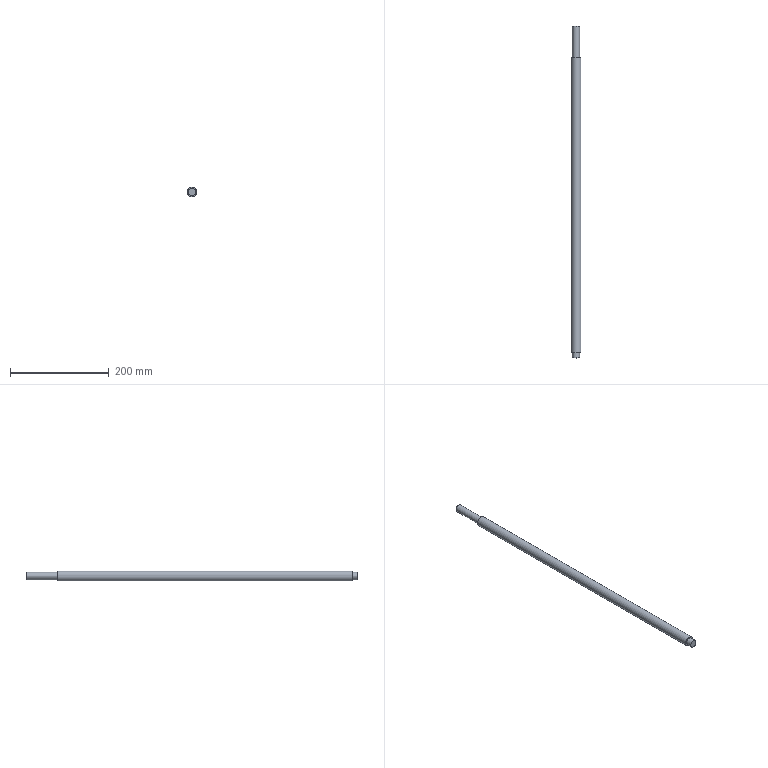Part | STEP file | tulunzhou | 1 solid | 7 faces | box 20 x 672 x 20 mm | volume 200669 mm3 | plane 4 | cylinder 3 | commonest cylinder face diameters 15 x2 20 x1
STEP:
#1=CARTESIAN_POINT('',(0.,0.,0.));
#2=DIRECTION('',(0.,0.,1.));
#3=DIRECTION('',(1.,0.,0.));
#4=AXIS2_PLACEMENT_3D('',#1,#2,#3);
#5=CARTESIAN_POINT('',(0.,12.,7.5));
#6=VERTEX_POINT('',#5);
#7=CARTESIAN_POINT('',(0.,12.,0.));
#8=DIRECTION('',(0.,1.,0.));
#9=DIRECTION('',(0.,0.,1.));
#10=AXIS2_PLACEMENT_3D('',#7,#8,#9);
#11=CIRCLE('',#10,7.5);
#12=CARTESIAN_POINT('',(0.,12.,0.));
#13=DIRECTION('',(0.,-1.,0.));
#14=DIRECTION('',(0.,0.,-1.));
#15=AXIS2_PLACEMENT_3D('',#12,#13,#14);
#16=CYLINDRICAL_SURFACE('',#15,7.5);
#17=CARTESIAN_POINT('',(9.425,0.));
#18=DIRECTION('',(-1.,0.));
#19=VECTOR('',#18,1.);
#20=LINE('',#17,#19);
#21=(GEOMETRIC_REPRESENTATION_CONTEXT(2)PARAMETRIC_REPRESENTATION_CONTEXT()REPRESENTATION_CONTEXT('',''));
#22=DEFINITIONAL_REPRESENTATION('',(#20),#21);
#23=PCURVE('',#16,#22);
#24=CARTESIAN_POINT('',(0.,12.,0.));
#25=DIRECTION('',(0.,1.,0.));
#26=DIRECTION('',(0.,0.,1.));
#27=AXIS2_PLACEMENT_3D('',#24,#25,#26);
#28=PLANE('',#27);
#29=CARTESIAN_POINT('',(0.,0.));
#30=DIRECTION('',(1.,0.));
#31=AXIS2_PLACEMENT_2D('',#29,#30);
#32=CIRCLE('',#31,7.5);
#33=(GEOMETRIC_REPRESENTATION_CONTEXT(2)PARAMETRIC_REPRESENTATION_CONTEXT()REPRESENTATION_CONTEXT('',''));
#34=DEFINITIONAL_REPRESENTATION('',(#32),#33);
#35=PCURVE('',#28,#34);
#36=SURFACE_CURVE('',#11,(#23,#35),.PCURVE_S1.);
#37=EDGE_CURVE('',#6,#6,#36,.T.);
#38=ORIENTED_EDGE('',*,*,#37,.F.);
#39=CARTESIAN_POINT('',(0.,0.,7.5));
#40=VERTEX_POINT('',#39);
#41=CARTESIAN_POINT('',(0.,12.,7.5));
#42=CARTESIAN_POINT('',(0.,0.,7.5));
#43=B_SPLINE_CURVE_WITH_KNOTS('',1,(#41,#42),.UNSPECIFIED.,.F.,.F.,(2,2),(0.,12.),.PIECEWISE_BEZIER_KNOTS.);
#44=CARTESIAN_POINT('',(9.425,0.));
#45=DIRECTION('',(0.,1.));
#46=VECTOR('',#45,1.);
#47=LINE('',#44,#46);
#48=(GEOMETRIC_REPRESENTATION_CONTEXT(2)PARAMETRIC_REPRESENTATION_CONTEXT()REPRESENTATION_CONTEXT('',''));
#49=DEFINITIONAL_REPRESENTATION('',(#47),#48);
#50=PCURVE('',#16,#49);
#51=CARTESIAN_POINT('',(3.142,0.));
#52=DIRECTION('',(0.,1.));
#53=VECTOR('',#52,1.);
#54=LINE('',#51,#53);
#55=(GEOMETRIC_REPRESENTATION_CONTEXT(2)PARAMETRIC_REPRESENTATION_CONTEXT()REPRESENTATION_CONTEXT('',''));
#56=DEFINITIONAL_REPRESENTATION('',(#54),#55);
#57=PCURVE('',#16,#56);
#58=SEAM_CURVE('',#43,(#50,#57),.PCURVE_S1.);
#59=EDGE_CURVE('',#6,#40,#58,.T.);
#60=ORIENTED_EDGE('',*,*,#59,.T.);
#61=CARTESIAN_POINT('',(0.,0.,0.));
#62=DIRECTION('',(0.,1.,0.));
#63=DIRECTION('',(0.,0.,1.));
#64=AXIS2_PLACEMENT_3D('',#61,#62,#63);
#65=CIRCLE('',#64,7.5);
#66=CARTESIAN_POINT('',(9.425,12.));
#67=DIRECTION('',(-1.,0.));
#68=VECTOR('',#67,1.);
#69=LINE('',#66,#68);
#70=(GEOMETRIC_REPRESENTATION_CONTEXT(2)PARAMETRIC_REPRESENTATION_CONTEXT()REPRESENTATION_CONTEXT('',''));
#71=DEFINITIONAL_REPRESENTATION('',(#69),#70);
#72=PCURVE('',#16,#71);
#73=CARTESIAN_POINT('',(0.,0.,0.));
#74=DIRECTION('',(0.,1.,0.));
#75=DIRECTION('',(0.,0.,1.));
#76=AXIS2_PLACEMENT_3D('',#73,#74,#75);
#77=PLANE('',#76);
#78=CARTESIAN_POINT('',(0.,0.));
#79=DIRECTION('',(1.,0.));
#80=AXIS2_PLACEMENT_2D('',#78,#79);
#81=CIRCLE('',#80,7.5);
#82=(GEOMETRIC_REPRESENTATION_CONTEXT(2)PARAMETRIC_REPRESENTATION_CONTEXT()REPRESENTATION_CONTEXT('',''));
#83=DEFINITIONAL_REPRESENTATION('',(#81),#82);
#84=PCURVE('',#77,#83);
#85=SURFACE_CURVE('',#65,(#72,#84),.PCURVE_S1.);
#86=EDGE_CURVE('',#40,#40,#85,.T.);
#87=ORIENTED_EDGE('',*,*,#86,.T.);
#88=ORIENTED_EDGE('',*,*,#59,.F.);
#89=EDGE_LOOP('',(#38,#60,#87,#88));
#90=FACE_BOUND('',#89,.T.);
#91=ADVANCED_FACE('',(#90),#16,.T.);
#92=ORIENTED_EDGE('',*,*,#86,.F.);
#93=EDGE_LOOP('',(#92));
#94=FACE_BOUND('',#93,.T.);
#95=ADVANCED_FACE('',(#94),#77,.F.);
#96=CARTESIAN_POINT('',(0.,608.,10.));
#97=VERTEX_POINT('',#96);
#98=CARTESIAN_POINT('',(0.,608.,0.));
#99=DIRECTION('',(0.,1.,0.));
#100=DIRECTION('',(0.,0.,1.));
#101=AXIS2_PLACEMENT_3D('',#98,#99,#100);
#102=CIRCLE('',#101,10.);
#103=CARTESIAN_POINT('',(0.,608.,0.));
#104=DIRECTION('',(0.,-1.,0.));
#105=DIRECTION('',(0.,0.,-1.));
#106=AXIS2_PLACEMENT_3D('',#103,#104,#105);
#107=CYLINDRICAL_SURFACE('',#106,10.);
#108=CARTESIAN_POINT('',(9.425,0.));
#109=DIRECTION('',(-1.,0.));
#110=VECTOR('',#109,1.);
#111=LINE('',#108,#110);
#112=(GEOMETRIC_REPRESENTATION_CONTEXT(2)PARAMETRIC_REPRESENTATION_CONTEXT()REPRESENTATION_CONTEXT('',''));
#113=DEFINITIONAL_REPRESENTATION('',(#111),#112);
#114=PCURVE('',#107,#113);
#115=CARTESIAN_POINT('',(0.,608.,0.));
#116=DIRECTION('',(0.,1.,0.));
#117=DIRECTION('',(0.,0.,1.));
#118=AXIS2_PLACEMENT_3D('',#115,#116,#117);
#119=PLANE('',#118);
#120=CARTESIAN_POINT('',(0.,0.));
#121=DIRECTION('',(1.,0.));
#122=AXIS2_PLACEMENT_2D('',#120,#121);
#123=CIRCLE('',#122,10.);
#124=(GEOMETRIC_REPRESENTATION_CONTEXT(2)PARAMETRIC_REPRESENTATION_CONTEXT()REPRESENTATION_CONTEXT('',''));
#125=DEFINITIONAL_REPRESENTATION('',(#123),#124);
#126=PCURVE('',#119,#125);
#127=SURFACE_CURVE('',#102,(#114,#126),.PCURVE_S1.);
#128=EDGE_CURVE('',#97,#97,#127,.T.);
#129=ORIENTED_EDGE('',*,*,#128,.F.);
#130=CARTESIAN_POINT('',(0.,12.,10.));
#131=VERTEX_POINT('',#130);
#132=CARTESIAN_POINT('',(0.,608.,10.));
#133=CARTESIAN_POINT('',(0.,12.,10.));
#134=B_SPLINE_CURVE_WITH_KNOTS('',1,(#132,#133),.UNSPECIFIED.,.F.,.F.,(2,2),(0.,596.),.PIECEWISE_BEZIER_KNOTS.);
#135=CARTESIAN_POINT('',(9.425,0.));
#136=DIRECTION('',(0.,1.));
#137=VECTOR('',#136,1.);
#138=LINE('',#135,#137);
#139=(GEOMETRIC_REPRESENTATION_CONTEXT(2)PARAMETRIC_REPRESENTATION_CONTEXT()REPRESENTATION_CONTEXT('',''));
#140=DEFINITIONAL_REPRESENTATION('',(#138),#139);
#141=PCURVE('',#107,#140);
#142=CARTESIAN_POINT('',(3.142,0.));
#143=DIRECTION('',(0.,1.));
#144=VECTOR('',#143,1.);
#145=LINE('',#142,#144);
#146=(GEOMETRIC_REPRESENTATION_CONTEXT(2)PARAMETRIC_REPRESENTATION_CONTEXT()REPRESENTATION_CONTEXT('',''));
#147=DEFINITIONAL_REPRESENTATION('',(#145),#146);
#148=PCURVE('',#107,#147);
#149=SEAM_CURVE('',#134,(#141,#148),.PCURVE_S1.);
#150=EDGE_CURVE('',#97,#131,#149,.T.);
#151=ORIENTED_EDGE('',*,*,#150,.T.);
#152=CARTESIAN_POINT('',(0.,12.,0.));
#153=DIRECTION('',(0.,1.,0.));
#154=DIRECTION('',(0.,0.,1.));
#155=AXIS2_PLACEMENT_3D('',#152,#153,#154);
#156=CIRCLE('',#155,10.);
#157=CARTESIAN_POINT('',(9.425,596.));
#158=DIRECTION('',(-1.,0.));
#159=VECTOR('',#158,1.);
#160=LINE('',#157,#159);
#161=(GEOMETRIC_REPRESENTATION_CONTEXT(2)PARAMETRIC_REPRESENTATION_CONTEXT()REPRESENTATION_CONTEXT('',''));
#162=DEFINITIONAL_REPRESENTATION('',(#160),#161);
#163=PCURVE('',#107,#162);
#164=CARTESIAN_POINT('',(0.,0.));
#165=DIRECTION('',(1.,0.));
#166=AXIS2_PLACEMENT_2D('',#164,#165);
#167=CIRCLE('',#166,10.);
#168=(GEOMETRIC_REPRESENTATION_CONTEXT(2)PARAMETRIC_REPRESENTATION_CONTEXT()REPRESENTATION_CONTEXT('',''));
#169=DEFINITIONAL_REPRESENTATION('',(#167),#168);
#170=PCURVE('',#28,#169);
#171=SURFACE_CURVE('',#156,(#163,#170),.PCURVE_S1.);
#172=EDGE_CURVE('',#131,#131,#171,.T.);
#173=ORIENTED_EDGE('',*,*,#172,.T.);
#174=ORIENTED_EDGE('',*,*,#150,.F.);
#175=EDGE_LOOP('',(#129,#151,#173,#174));
#176=FACE_BOUND('',#175,.T.);
#177=ADVANCED_FACE('',(#176),#107,.T.);
#178=CARTESIAN_POINT('',(0.,608.,7.5));
#179=VERTEX_POINT('',#178);
#180=CARTESIAN_POINT('',(0.,608.,0.));
#181=DIRECTION('',(0.,1.,0.));
#182=DIRECTION('',(0.,0.,1.));
#183=AXIS2_PLACEMENT_3D('',#180,#181,#182);
#184=CIRCLE('',#183,7.5);
#185=CARTESIAN_POINT('',(0.,0.));
#186=DIRECTION('',(1.,0.));
#187=AXIS2_PLACEMENT_2D('',#185,#186);
#188=CIRCLE('',#187,7.5);
#189=(GEOMETRIC_REPRESENTATION_CONTEXT(2)PARAMETRIC_REPRESENTATION_CONTEXT()REPRESENTATION_CONTEXT('',''));
#190=DEFINITIONAL_REPRESENTATION('',(#188),#189);
#191=PCURVE('',#119,#190);
#192=CARTESIAN_POINT('',(0.,672.,0.));
#193=DIRECTION('',(0.,-1.,0.));
#194=DIRECTION('',(0.,0.,-1.));
#195=AXIS2_PLACEMENT_3D('',#192,#193,#194);
#196=CYLINDRICAL_SURFACE('',#195,7.5);
#197=CARTESIAN_POINT('',(9.425,64.));
#198=DIRECTION('',(-1.,0.));
#199=VECTOR('',#198,1.);
#200=LINE('',#197,#199);
#201=(GEOMETRIC_REPRESENTATION_CONTEXT(2)PARAMETRIC_REPRESENTATION_CONTEXT()REPRESENTATION_CONTEXT('',''));
#202=DEFINITIONAL_REPRESENTATION('',(#200),#201);
#203=PCURVE('',#196,#202);
#204=SURFACE_CURVE('',#184,(#191,#203),.PCURVE_S1.);
#205=EDGE_CURVE('',#179,#179,#204,.T.);
#206=ORIENTED_EDGE('',*,*,#205,.F.);
#207=EDGE_LOOP('',(#206));
#208=FACE_BOUND('',#207,.T.);
#209=ORIENTED_EDGE('',*,*,#128,.T.);
#210=EDGE_LOOP('',(#209));
#211=FACE_BOUND('',#210,.T.);
#212=ADVANCED_FACE('',(#208,#211),#119,.T.);
#213=ORIENTED_EDGE('',*,*,#37,.T.);
#214=EDGE_LOOP('',(#213));
#215=FACE_BOUND('',#214,.T.);
#216=ORIENTED_EDGE('',*,*,#172,.F.);
#217=EDGE_LOOP('',(#216));
#218=FACE_BOUND('',#217,.T.);
#219=ADVANCED_FACE('',(#215,#218),#28,.F.);
#220=CARTESIAN_POINT('',(0.,672.,7.5));
#221=VERTEX_POINT('',#220);
#222=CARTESIAN_POINT('',(0.,672.,0.));
#223=DIRECTION('',(0.,1.,0.));
#224=DIRECTION('',(0.,0.,1.));
#225=AXIS2_PLACEMENT_3D('',#222,#223,#224);
#226=CIRCLE('',#225,7.5);
#227=CARTESIAN_POINT('',(9.425,0.));
#228=DIRECTION('',(-1.,0.));
#229=VECTOR('',#228,1.);
#230=LINE('',#227,#229);
#231=(GEOMETRIC_REPRESENTATION_CONTEXT(2)PARAMETRIC_REPRESENTATION_CONTEXT()REPRESENTATION_CONTEXT('',''));
#232=DEFINITIONAL_REPRESENTATION('',(#230),#231);
#233=PCURVE('',#196,#232);
#234=CARTESIAN_POINT('',(0.,672.,0.));
#235=DIRECTION('',(0.,1.,0.));
#236=DIRECTION('',(0.,0.,1.));
#237=AXIS2_PLACEMENT_3D('',#234,#235,#236);
#238=PLANE('',#237);
#239=CARTESIAN_POINT('',(0.,0.));
#240=DIRECTION('',(1.,0.));
#241=AXIS2_PLACEMENT_2D('',#239,#240);
#242=CIRCLE('',#241,7.5);
#243=(GEOMETRIC_REPRESENTATION_CONTEXT(2)PARAMETRIC_REPRESENTATION_CONTEXT()REPRESENTATION_CONTEXT('',''));
#244=DEFINITIONAL_REPRESENTATION('',(#242),#243);
#245=PCURVE('',#238,#244);
#246=SURFACE_CURVE('',#226,(#233,#245),.PCURVE_S1.);
#247=EDGE_CURVE('',#221,#221,#246,.T.);
#248=ORIENTED_EDGE('',*,*,#247,.F.);
#249=CARTESIAN_POINT('',(0.,672.,7.5));
#250=CARTESIAN_POINT('',(0.,608.,7.5));
#251=B_SPLINE_CURVE_WITH_KNOTS('',1,(#249,#250),.UNSPECIFIED.,.F.,.F.,(2,2),(0.,64.),.PIECEWISE_BEZIER_KNOTS.);
#252=CARTESIAN_POINT('',(9.425,0.));
#253=DIRECTION('',(0.,1.));
#254=VECTOR('',#253,1.);
#255=LINE('',#252,#254);
#256=(GEOMETRIC_REPRESENTATION_CONTEXT(2)PARAMETRIC_REPRESENTATION_CONTEXT()REPRESENTATION_CONTEXT('',''));
#257=DEFINITIONAL_REPRESENTATION('',(#255),#256);
#258=PCURVE('',#196,#257);
#259=CARTESIAN_POINT('',(3.142,0.));
#260=DIRECTION('',(0.,1.));
#261=VECTOR('',#260,1.);
#262=LINE('',#259,#261);
#263=(GEOMETRIC_REPRESENTATION_CONTEXT(2)PARAMETRIC_REPRESENTATION_CONTEXT()REPRESENTATION_CONTEXT('',''));
#264=DEFINITIONAL_REPRESENTATION('',(#262),#263);
#265=PCURVE('',#196,#264);
#266=SEAM_CURVE('',#251,(#258,#265),.PCURVE_S1.);
#267=EDGE_CURVE('',#221,#179,#266,.T.);
#268=ORIENTED_EDGE('',*,*,#267,.T.);
#269=ORIENTED_EDGE('',*,*,#205,.T.);
#270=ORIENTED_EDGE('',*,*,#267,.F.);
#271=EDGE_LOOP('',(#248,#268,#269,#270));
#272=FACE_BOUND('',#271,.T.);
#273=ADVANCED_FACE('',(#272),#196,.T.);
#274=ORIENTED_EDGE('',*,*,#247,.T.);
#275=EDGE_LOOP('',(#274));
#276=FACE_BOUND('',#275,.T.);
#277=ADVANCED_FACE('',(#276),#238,.T.);
#278=CLOSED_SHELL('',(#91,#95,#177,#212,#219,#273,#277));
#279=MANIFOLD_SOLID_BREP('',#278);
#280=(LENGTH_UNIT()NAMED_UNIT(*)SI_UNIT(.MILLI.,.METRE.));
#281=UNCERTAINTY_MEASURE_WITH_UNIT(LENGTH_MEASURE(0.00001),#280,'','');
#282=(NAMED_UNIT(*)PLANE_ANGLE_UNIT()SI_UNIT($,.RADIAN.));
#283=(NAMED_UNIT(*)SI_UNIT($,.STERADIAN.)SOLID_ANGLE_UNIT());
#284=(GEOMETRIC_REPRESENTATION_CONTEXT(3)GLOBAL_UNCERTAINTY_ASSIGNED_CONTEXT((#281))GLOBAL_UNIT_ASSIGNED_CONTEXT((#280,#282,#283))REPRESENTATION_CONTEXT('',''));
#285=ADVANCED_BREP_SHAPE_REPRESENTATION('',(#4,#279),#284);